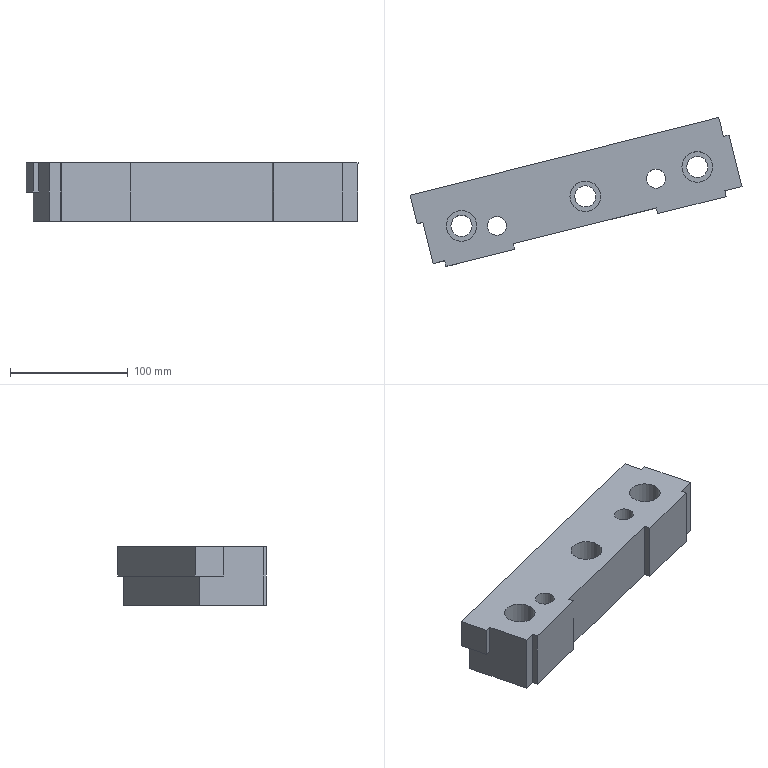Part | NX | features solid 2 | 1 solid | 31 faces | box 281.581 x 126.317 x 50 mm | volume 740203 mm3 | plane 20 | cylinder 8 | spline 3 | commonest cylinder face diameters 18 x3 26 x3 16 x2
STEP:
#1=CARTESIAN_POINT('',(-1.015,507.696,-50.));
#2=VERTEX_POINT('',#1);
#3=CARTESIAN_POINT('',(-10.015,507.696,-50.));
#4=DIRECTION('',(0.,0.,1.));
#5=DIRECTION('',(1.,0.,0.));
#6=AXIS2_PLACEMENT_3D('',#3,#4,#5);
#7=CIRCLE('',#6,9.);
#8=EDGE_CURVE('',#2,#2,#7,.T.);
#9=ORIENTED_EDGE('',*,*,#8,.F.);
#10=EDGE_LOOP('',(#9));
#11=FACE_BOUND('',#10,.T.);
#12=CARTESIAN_POINT('',(-1.015,507.696,-30.));
#13=VERTEX_POINT('',#12);
#14=CARTESIAN_POINT('',(-10.015,507.696,-30.));
#15=DIRECTION('',(0.,0.,1.));
#16=DIRECTION('',(1.,0.,0.));
#17=AXIS2_PLACEMENT_3D('',#14,#15,#16);
#18=CIRCLE('',#17,9.);
#19=EDGE_CURVE('',#13,#13,#18,.F.);
#20=ORIENTED_EDGE('',*,*,#19,.F.);
#21=EDGE_LOOP('',(#20));
#22=FACE_BOUND('',#21,.T.);
#23=CARTESIAN_POINT('',(-10.015,507.696,-125.));
#24=DIRECTION('',(0.,0.,1.));
#25=DIRECTION('',(1.,0.,0.));
#26=AXIS2_PLACEMENT_3D('',#23,#24,#25);
#27=CYLINDRICAL_SURFACE('',#26,9.);
#28=ADVANCED_FACE('',(#11,#22),#27,.F.);
#29=CARTESIAN_POINT('',(103.985,532.696,-50.));
#30=VERTEX_POINT('',#29);
#31=CARTESIAN_POINT('',(94.985,532.696,-50.));
#32=DIRECTION('',(0.,0.,1.));
#33=DIRECTION('',(1.,0.,0.));
#34=AXIS2_PLACEMENT_3D('',#31,#32,#33);
#35=CIRCLE('',#34,9.);
#36=EDGE_CURVE('',#30,#30,#35,.T.);
#37=ORIENTED_EDGE('',*,*,#36,.F.);
#38=EDGE_LOOP('',(#37));
#39=FACE_BOUND('',#38,.T.);
#40=CARTESIAN_POINT('',(103.985,532.696,-30.));
#41=VERTEX_POINT('',#40);
#42=CARTESIAN_POINT('',(94.985,532.696,-30.));
#43=DIRECTION('',(0.,0.,1.));
#44=DIRECTION('',(1.,0.,0.));
#45=AXIS2_PLACEMENT_3D('',#42,#43,#44);
#46=CIRCLE('',#45,9.);
#47=EDGE_CURVE('',#41,#41,#46,.F.);
#48=ORIENTED_EDGE('',*,*,#47,.F.);
#49=EDGE_LOOP('',(#48));
#50=FACE_BOUND('',#49,.T.);
#51=CARTESIAN_POINT('',(94.985,532.696,-125.));
#52=DIRECTION('',(0.,0.,1.));
#53=DIRECTION('',(1.,0.,0.));
#54=AXIS2_PLACEMENT_3D('',#51,#52,#53);
#55=CYLINDRICAL_SURFACE('',#54,9.);
#56=ADVANCED_FACE('',(#39,#50),#55,.F.);
#57=CARTESIAN_POINT('',(198.985,557.696,-50.));
#58=VERTEX_POINT('',#57);
#59=CARTESIAN_POINT('',(189.985,557.696,-50.));
#60=DIRECTION('',(0.,0.,1.));
#61=DIRECTION('',(1.,0.,0.));
#62=AXIS2_PLACEMENT_3D('',#59,#60,#61);
#63=CIRCLE('',#62,9.);
#64=EDGE_CURVE('',#58,#58,#63,.T.);
#65=ORIENTED_EDGE('',*,*,#64,.F.);
#66=EDGE_LOOP('',(#65));
#67=FACE_BOUND('',#66,.T.);
#68=CARTESIAN_POINT('',(198.985,557.696,-30.));
#69=VERTEX_POINT('',#68);
#70=CARTESIAN_POINT('',(189.985,557.696,-30.));
#71=DIRECTION('',(0.,0.,1.));
#72=DIRECTION('',(1.,0.,0.));
#73=AXIS2_PLACEMENT_3D('',#70,#71,#72);
#74=CIRCLE('',#73,9.);
#75=EDGE_CURVE('',#69,#69,#74,.F.);
#76=ORIENTED_EDGE('',*,*,#75,.F.);
#77=EDGE_LOOP('',(#76));
#78=FACE_BOUND('',#77,.T.);
#79=CARTESIAN_POINT('',(189.985,557.696,-125.));
#80=DIRECTION('',(0.,0.,1.));
#81=DIRECTION('',(1.,0.,0.));
#82=AXIS2_PLACEMENT_3D('',#79,#80,#81);
#83=CYLINDRICAL_SURFACE('',#82,9.);
#84=ADVANCED_FACE('',(#67,#78),#83,.F.);
#85=CARTESIAN_POINT('',(155.109,522.891,0.));
#86=VERTEX_POINT('',#85);
#87=CARTESIAN_POINT('',(155.109,522.891,-50.));
#88=VERTEX_POINT('',#87);
#89=CARTESIAN_POINT('',(155.109,522.891,-70.));
#90=DIRECTION('',(0.,0.,-1.));
#91=VECTOR('',#90,1000.);
#92=LINE('',#89,#91);
#93=EDGE_CURVE('',#86,#88,#92,.T.);
#94=ORIENTED_EDGE('',*,*,#93,.F.);
#95=CARTESIAN_POINT('',(33.822,492.651,0.));
#96=VERTEX_POINT('',#95);
#97=CARTESIAN_POINT('',(-300.93,409.188,0.));
#98=DIRECTION('',(-0.9703,-0.2419,0.));
#99=VECTOR('',#98,1000.);
#100=LINE('',#97,#99);
#101=EDGE_CURVE('',#86,#96,#100,.T.);
#102=ORIENTED_EDGE('',*,*,#101,.T.);
#103=CARTESIAN_POINT('',(33.822,492.651,-50.));
#104=VERTEX_POINT('',#103);
#105=CARTESIAN_POINT('',(33.822,492.651,-70.));
#106=DIRECTION('',(0.,0.,-1.));
#107=VECTOR('',#106,1000.);
#108=LINE('',#105,#107);
#109=EDGE_CURVE('',#96,#104,#108,.T.);
#110=ORIENTED_EDGE('',*,*,#109,.T.);
#111=CARTESIAN_POINT('',(-232.339,426.29,-50.));
#112=DIRECTION('',(0.9703,0.2419,0.));
#113=VECTOR('',#112,1000.);
#114=LINE('',#111,#113);
#115=EDGE_CURVE('',#104,#88,#114,.T.);
#116=ORIENTED_EDGE('',*,*,#115,.T.);
#117=EDGE_LOOP('',(#94,#102,#110,#116));
#118=FACE_BOUND('',#117,.T.);
#119=CARTESIAN_POINT('',(-300.93,409.188,-70.));
#120=DIRECTION('',(0.2419,-0.9703,0.));
#121=DIRECTION('',(0.9703,0.2419,0.));
#122=AXIS2_PLACEMENT_3D('',#119,#120,#121);
#123=PLANE('',#122);
#124=ADVANCED_FACE('',(#118),#123,.T.);
#125=CARTESIAN_POINT('',(212.143,583.489,0.));
#126=VERTEX_POINT('',#125);
#127=CARTESIAN_POINT('',(216.994,584.699,0.));
#128=VERTEX_POINT('',#127);
#129=CARTESIAN_POINT('',(212.143,583.489,0.));
#130=DIRECTION('',(0.9703,0.2419,0.));
#131=VECTOR('',#130,1000.);
#132=LINE('',#129,#131);
#133=EDGE_CURVE('',#126,#128,#132,.T.);
#134=ORIENTED_EDGE('',*,*,#133,.F.);
#135=CARTESIAN_POINT('',(208.125,599.602,0.));
#136=VERTEX_POINT('',#135);
#137=CARTESIAN_POINT('',(537.993,-723.425,0.));
#138=DIRECTION('',(-0.2419,0.9703,0.));
#139=VECTOR('',#138,1000.);
#140=LINE('',#137,#139);
#141=EDGE_CURVE('',#126,#136,#140,.T.);
#142=ORIENTED_EDGE('',*,*,#141,.T.);
#143=CARTESIAN_POINT('',(-53.7,533.663,0.));
#144=VERTEX_POINT('',#143);
#145=CARTESIAN_POINT('',(208.125,599.602,0.));
#146=CARTESIAN_POINT('',(120.85,577.623,0.));
#147=CARTESIAN_POINT('',(33.576,555.638,0.));
#148=CARTESIAN_POINT('',(-53.7,533.663,0.));
#149=B_SPLINE_CURVE_WITH_KNOTS('',3,(#145,#146,#147,#148),.UNSPECIFIED.,.F.,.F.,(4,4),(1.862,2.132),.UNSPECIFIED.);
#150=EDGE_CURVE('',#144,#136,#149,.F.);
#151=ORIENTED_EDGE('',*,*,#150,.F.);
#152=CARTESIAN_POINT('',(-47.652,509.406,0.));
#153=VERTEX_POINT('',#152);
#154=CARTESIAN_POINT('',(276.013,-788.744,0.));
#155=DIRECTION('',(-0.2419,0.9703,0.));
#156=VECTOR('',#155,1000.);
#157=LINE('',#154,#156);
#158=EDGE_CURVE('',#153,#144,#157,.T.);
#159=ORIENTED_EDGE('',*,*,#158,.F.);
#160=CARTESIAN_POINT('',(-42.803,510.627,0.));
#161=VERTEX_POINT('',#160);
#162=CARTESIAN_POINT('',(-47.652,509.406,0.));
#163=CARTESIAN_POINT('',(-46.036,509.813,0.));
#164=CARTESIAN_POINT('',(-44.419,510.22,0.));
#165=CARTESIAN_POINT('',(-42.803,510.627,0.));
#166=B_SPLINE_CURVE_WITH_KNOTS('',3,(#162,#163,#164,#165),.UNSPECIFIED.,.F.,.F.,(4,4),(0.,0.005),.UNSPECIFIED.);
#167=EDGE_CURVE('',#153,#161,#166,.T.);
#168=ORIENTED_EDGE('',*,*,#167,.T.);
#169=CARTESIAN_POINT('',(-34.099,475.717,0.));
#170=VERTEX_POINT('',#169);
#171=CARTESIAN_POINT('',(-23.213,432.053,0.));
#172=DIRECTION('',(0.2419,-0.9703,0.));
#173=VECTOR('',#172,1000.);
#174=LINE('',#171,#173);
#175=EDGE_CURVE('',#161,#170,#174,.T.);
#176=ORIENTED_EDGE('',*,*,#175,.T.);
#177=CARTESIAN_POINT('',(-24.396,478.136,0.));
#178=VERTEX_POINT('',#177);
#179=CARTESIAN_POINT('',(-300.93,409.188,0.));
#180=DIRECTION('',(-0.9703,-0.2419,0.));
#181=VECTOR('',#180,1000.);
#182=LINE('',#179,#181);
#183=EDGE_CURVE('',#178,#170,#182,.T.);
#184=ORIENTED_EDGE('',*,*,#183,.F.);
#185=CARTESIAN_POINT('',(-23.187,473.284,0.));
#186=VERTEX_POINT('',#185);
#187=CARTESIAN_POINT('',(-39.146,537.292,0.));
#188=DIRECTION('',(0.2419,-0.9703,0.));
#189=VECTOR('',#188,1000.);
#190=LINE('',#187,#189);
#191=EDGE_CURVE('',#178,#186,#190,.T.);
#192=ORIENTED_EDGE('',*,*,#191,.T.);
#193=CARTESIAN_POINT('',(35.031,487.8,0.));
#194=VERTEX_POINT('',#193);
#195=CARTESIAN_POINT('',(-231.129,421.438,0.));
#196=DIRECTION('',(0.9703,0.2419,0.));
#197=VECTOR('',#196,1000.);
#198=LINE('',#195,#197);
#199=EDGE_CURVE('',#186,#194,#198,.T.);
#200=ORIENTED_EDGE('',*,*,#199,.T.);
#201=CARTESIAN_POINT('',(19.072,551.808,0.));
#202=DIRECTION('',(0.2419,-0.9703,0.));
#203=VECTOR('',#202,1000.);
#204=LINE('',#201,#203);
#205=EDGE_CURVE('',#96,#194,#204,.T.);
#206=ORIENTED_EDGE('',*,*,#205,.F.);
#207=ORIENTED_EDGE('',*,*,#101,.F.);
#208=CARTESIAN_POINT('',(156.318,518.04,0.));
#209=VERTEX_POINT('',#208);
#210=CARTESIAN_POINT('',(140.359,582.048,0.));
#211=DIRECTION('',(0.2419,-0.9703,0.));
#212=VECTOR('',#211,1000.);
#213=LINE('',#210,#212);
#214=EDGE_CURVE('',#86,#209,#213,.T.);
#215=ORIENTED_EDGE('',*,*,#214,.T.);
#216=CARTESIAN_POINT('',(214.536,532.555,0.));
#217=VERTEX_POINT('',#216);
#218=CARTESIAN_POINT('',(-231.129,421.438,0.));
#219=DIRECTION('',(0.9703,0.2419,0.));
#220=VECTOR('',#219,1000.);
#221=LINE('',#218,#220);
#222=EDGE_CURVE('',#209,#217,#221,.T.);
#223=ORIENTED_EDGE('',*,*,#222,.T.);
#224=CARTESIAN_POINT('',(213.326,537.407,0.));
#225=VERTEX_POINT('',#224);
#226=CARTESIAN_POINT('',(198.577,596.563,0.));
#227=DIRECTION('',(0.2419,-0.9703,0.));
#228=VECTOR('',#227,1000.);
#229=LINE('',#226,#228);
#230=EDGE_CURVE('',#225,#217,#229,.T.);
#231=ORIENTED_EDGE('',*,*,#230,.F.);
#232=CARTESIAN_POINT('',(227.881,541.035,0.));
#233=VERTEX_POINT('',#232);
#234=CARTESIAN_POINT('',(-232.339,426.29,0.));
#235=DIRECTION('',(-0.9703,-0.2419,0.));
#236=VECTOR('',#235,1000.);
#237=LINE('',#234,#236);
#238=EDGE_CURVE('',#233,#225,#237,.T.);
#239=ORIENTED_EDGE('',*,*,#238,.F.);
#240=CARTESIAN_POINT('',(237.558,502.224,0.));
#241=DIRECTION('',(-0.2419,0.9703,0.));
#242=VECTOR('',#241,1000.);
#243=LINE('',#240,#242);
#244=EDGE_CURVE('',#233,#128,#243,.T.);
#245=ORIENTED_EDGE('',*,*,#244,.T.);
#246=EDGE_LOOP('',(#134,#142,#151,#159,#168,#176,#184,#192,#200,#206,#207,#215,#223,#231,#239,#245));
#247=FACE_BOUND('',#246,.T.);
#248=CARTESIAN_POINT('',(2.985,507.696,0.));
#249=VERTEX_POINT('',#248);
#250=CARTESIAN_POINT('',(-10.015,507.696,0.));
#251=DIRECTION('',(0.,0.,1.));
#252=DIRECTION('',(1.,0.,0.));
#253=AXIS2_PLACEMENT_3D('',#250,#251,#252);
#254=CIRCLE('',#253,13.);
#255=EDGE_CURVE('',#249,#249,#254,.T.);
#256=ORIENTED_EDGE('',*,*,#255,.F.);
#257=EDGE_LOOP('',(#256));
#258=FACE_BOUND('',#257,.T.);
#259=CARTESIAN_POINT('',(107.985,532.696,0.));
#260=VERTEX_POINT('',#259);
#261=CARTESIAN_POINT('',(94.985,532.696,0.));
#262=DIRECTION('',(0.,0.,1.));
#263=DIRECTION('',(1.,0.,0.));
#264=AXIS2_PLACEMENT_3D('',#261,#262,#263);
#265=CIRCLE('',#264,13.);
#266=EDGE_CURVE('',#260,#260,#265,.T.);
#267=ORIENTED_EDGE('',*,*,#266,.F.);
#268=EDGE_LOOP('',(#267));
#269=FACE_BOUND('',#268,.T.);
#270=CARTESIAN_POINT('',(202.985,557.696,0.));
#271=VERTEX_POINT('',#270);
#272=CARTESIAN_POINT('',(189.985,557.696,0.));
#273=DIRECTION('',(0.,0.,1.));
#274=DIRECTION('',(1.,0.,0.));
#275=AXIS2_PLACEMENT_3D('',#272,#273,#274);
#276=CIRCLE('',#275,13.);
#277=EDGE_CURVE('',#271,#271,#276,.T.);
#278=ORIENTED_EDGE('',*,*,#277,.F.);
#279=EDGE_LOOP('',(#278));
#280=FACE_BOUND('',#279,.T.);
#281=CARTESIAN_POINT('',(27.985,507.696,0.));
#282=VERTEX_POINT('',#281);
#283=CARTESIAN_POINT('',(19.985,507.696,0.));
#284=DIRECTION('',(0.,0.,1.));
#285=DIRECTION('',(1.,0.,0.));
#286=AXIS2_PLACEMENT_3D('',#283,#284,#285);
#287=CIRCLE('',#286,8.);
#288=EDGE_CURVE('',#282,#282,#287,.T.);
#289=ORIENTED_EDGE('',*,*,#288,.F.);
#290=EDGE_LOOP('',(#289));
#291=FACE_BOUND('',#290,.T.);
#292=CARTESIAN_POINT('',(162.985,547.696,0.));
#293=VERTEX_POINT('',#292);
#294=CARTESIAN_POINT('',(154.985,547.696,0.));
#295=DIRECTION('',(0.,0.,1.));
#296=DIRECTION('',(1.,0.,0.));
#297=AXIS2_PLACEMENT_3D('',#294,#295,#296);
#298=CIRCLE('',#297,8.);
#299=EDGE_CURVE('',#293,#293,#298,.T.);
#300=ORIENTED_EDGE('',*,*,#299,.F.);
#301=EDGE_LOOP('',(#300));
#302=FACE_BOUND('',#301,.T.);
#303=CARTESIAN_POINT('',(82.625,-836.961,0.));
#304=DIRECTION('',(0.,0.,1.));
#305=DIRECTION('',(1.,0.,0.));
#306=AXIS2_PLACEMENT_3D('',#303,#304,#305);
#307=PLANE('',#306);
#308=ADVANCED_FACE('',(#247,#258,#269,#280,#291,#302),#307,.T.);
#309=CARTESIAN_POINT('',(-47.652,509.406,-25.));
#310=VERTEX_POINT('',#309);
#311=CARTESIAN_POINT('',(-42.803,510.627,-25.));
#312=VERTEX_POINT('',#311);
#313=CARTESIAN_POINT('',(-47.652,509.406,-25.));
#314=CARTESIAN_POINT('',(-46.036,509.813,-25.));
#315=CARTESIAN_POINT('',(-44.419,510.22,-25.));
#316=CARTESIAN_POINT('',(-42.803,510.627,-25.));
#317=B_SPLINE_CURVE_WITH_KNOTS('',3,(#313,#314,#315,#316),.UNSPECIFIED.,.F.,.F.,(4,4),(-0.0002137,0.01831),.UNSPECIFIED.);
#318=EDGE_CURVE('',#310,#312,#317,.T.);
#319=ORIENTED_EDGE('',*,*,#318,.F.);
#320=CARTESIAN_POINT('',(-53.7,533.663,-25.));
#321=VERTEX_POINT('',#320);
#322=CARTESIAN_POINT('',(-53.7,533.663,-25.));
#323=DIRECTION('',(0.2419,-0.9703,0.));
#324=VECTOR('',#323,1000.);
#325=LINE('',#322,#324);
#326=EDGE_CURVE('',#321,#310,#325,.T.);
#327=ORIENTED_EDGE('',*,*,#326,.F.);
#328=CARTESIAN_POINT('',(208.125,599.602,-25.));
#329=VERTEX_POINT('',#328);
#330=CARTESIAN_POINT('',(208.125,599.602,-25.));
#331=CARTESIAN_POINT('',(120.85,577.623,-25.));
#332=CARTESIAN_POINT('',(33.576,555.638,-25.));
#333=CARTESIAN_POINT('',(-53.7,533.663,-25.));
#334=B_SPLINE_CURVE_WITH_KNOTS('',3,(#330,#331,#332,#333),.UNSPECIFIED.,.F.,.F.,(4,4),(1.907,2.177),.UNSPECIFIED.);
#335=EDGE_CURVE('',#321,#329,#334,.F.);
#336=ORIENTED_EDGE('',*,*,#335,.T.);
#337=CARTESIAN_POINT('',(209.335,594.75,-25.));
#338=VERTEX_POINT('',#337);
#339=CARTESIAN_POINT('',(820.536,-1856.645,-25.));
#340=DIRECTION('',(-0.2419,0.9703,0.));
#341=VECTOR('',#340,1000.);
#342=LINE('',#339,#341);
#343=EDGE_CURVE('',#338,#329,#342,.T.);
#344=ORIENTED_EDGE('',*,*,#343,.F.);
#345=CARTESIAN_POINT('',(-47.642,530.033,-25.));
#346=VERTEX_POINT('',#345);
#347=CARTESIAN_POINT('',(209.335,594.75,-25.));
#348=CARTESIAN_POINT('',(123.676,573.178,-25.));
#349=CARTESIAN_POINT('',(38.019,551.599,-25.));
#350=CARTESIAN_POINT('',(-47.642,530.033,-25.));
#351=B_SPLINE_CURVE_WITH_KNOTS('',3,(#347,#348,#349,#350),.UNSPECIFIED.,.F.,.F.,(4,4),(1.091,1.356),.UNSPECIFIED.);
#352=EDGE_CURVE('',#346,#338,#351,.F.);
#353=ORIENTED_EDGE('',*,*,#352,.F.);
#354=CARTESIAN_POINT('',(-23.213,432.053,-25.));
#355=DIRECTION('',(-0.2419,0.9703,0.));
#356=VECTOR('',#355,1000.);
#357=LINE('',#354,#356);
#358=EDGE_CURVE('',#312,#346,#357,.T.);
#359=ORIENTED_EDGE('',*,*,#358,.F.);
#360=EDGE_LOOP('',(#319,#327,#336,#344,#353,#359));
#361=FACE_BOUND('',#360,.T.);
#362=CARTESIAN_POINT('',(-53.7,533.663,-25.));
#363=DIRECTION('',(0.,0.,-1.));
#364=DIRECTION('',(-1.,0.,0.));
#365=AXIS2_PLACEMENT_3D('',#362,#363,#364);
#366=PLANE('',#365);
#367=ADVANCED_FACE('',(#361),#366,.T.);
#368=ORIENTED_EDGE('',*,*,#326,.T.);
#369=CARTESIAN_POINT('',(-47.652,509.406,-12.5));
#370=DIRECTION('',(0.,0.,-1.));
#371=VECTOR('',#370,1000.);
#372=LINE('',#369,#371);
#373=EDGE_CURVE('',#310,#153,#372,.F.);
#374=ORIENTED_EDGE('',*,*,#373,.T.);
#375=ORIENTED_EDGE('',*,*,#158,.T.);
#376=CARTESIAN_POINT('',(-53.7,533.663,-2.5));
#377=DIRECTION('',(0.,0.,1.));
#378=VECTOR('',#377,1000.);
#379=LINE('',#376,#378);
#380=EDGE_CURVE('',#321,#144,#379,.T.);
#381=ORIENTED_EDGE('',*,*,#380,.F.);
#382=EDGE_LOOP('',(#368,#374,#375,#381));
#383=FACE_BOUND('',#382,.T.);
#384=CARTESIAN_POINT('',(558.557,-1921.963,-70.));
#385=DIRECTION('',(0.9703,0.2419,0.));
#386=DIRECTION('',(-0.2419,0.9703,0.));
#387=AXIS2_PLACEMENT_3D('',#384,#385,#386);
#388=PLANE('',#387);
#389=ADVANCED_FACE('',(#383),#388,.F.);
#390=CARTESIAN_POINT('',(-24.396,478.136,-50.));
#391=VERTEX_POINT('',#390);
#392=CARTESIAN_POINT('',(-24.396,478.136,-70.));
#393=DIRECTION('',(0.,0.,-1.));
#394=VECTOR('',#393,1000.);
#395=LINE('',#392,#394);
#396=EDGE_CURVE('',#178,#391,#395,.T.);
#397=ORIENTED_EDGE('',*,*,#396,.F.);
#398=ORIENTED_EDGE('',*,*,#183,.T.);
#399=CARTESIAN_POINT('',(-34.099,475.717,-50.));
#400=VERTEX_POINT('',#399);
#401=CARTESIAN_POINT('',(-34.099,475.717,-70.));
#402=DIRECTION('',(0.,0.,1.));
#403=VECTOR('',#402,1000.);
#404=LINE('',#401,#403);
#405=EDGE_CURVE('',#400,#170,#404,.T.);
#406=ORIENTED_EDGE('',*,*,#405,.F.);
#407=CARTESIAN_POINT('',(-232.339,426.29,-50.));
#408=DIRECTION('',(0.9703,0.2419,0.));
#409=VECTOR('',#408,1000.);
#410=LINE('',#407,#409);
#411=EDGE_CURVE('',#400,#391,#410,.T.);
#412=ORIENTED_EDGE('',*,*,#411,.T.);
#413=EDGE_LOOP('',(#397,#398,#406,#412));
#414=FACE_BOUND('',#413,.T.);
#415=CARTESIAN_POINT('',(-300.93,409.188,-70.));
#416=DIRECTION('',(0.2419,-0.9703,0.));
#417=DIRECTION('',(0.9703,0.2419,0.));
#418=AXIS2_PLACEMENT_3D('',#415,#416,#417);
#419=PLANE('',#418);
#420=ADVANCED_FACE('',(#414),#419,.T.);
#421=CARTESIAN_POINT('',(212.143,583.489,-50.));
#422=VERTEX_POINT('',#421);
#423=CARTESIAN_POINT('',(212.143,583.489,-70.));
#424=DIRECTION('',(0.,0.,1.));
#425=VECTOR('',#424,1000.);
#426=LINE('',#423,#425);
#427=EDGE_CURVE('',#422,#126,#426,.T.);
#428=ORIENTED_EDGE('',*,*,#427,.F.);
#429=CARTESIAN_POINT('',(209.335,594.75,-50.));
#430=VERTEX_POINT('',#429);
#431=CARTESIAN_POINT('',(537.993,-723.425,-50.));
#432=DIRECTION('',(-0.2419,0.9703,0.));
#433=VECTOR('',#432,1000.);
#434=LINE('',#431,#433);
#435=EDGE_CURVE('',#422,#430,#434,.T.);
#436=ORIENTED_EDGE('',*,*,#435,.T.);
#437=CARTESIAN_POINT('',(209.335,594.75,-42.5));
#438=DIRECTION('',(0.,0.,1.));
#439=VECTOR('',#438,1000.);
#440=LINE('',#437,#439);
#441=EDGE_CURVE('',#338,#430,#440,.F.);
#442=ORIENTED_EDGE('',*,*,#441,.F.);
#443=ORIENTED_EDGE('',*,*,#343,.T.);
#444=CARTESIAN_POINT('',(208.125,599.602,-70.));
#445=DIRECTION('',(0.,0.,1.));
#446=VECTOR('',#445,1000.);
#447=LINE('',#444,#446);
#448=EDGE_CURVE('',#329,#136,#447,.T.);
#449=ORIENTED_EDGE('',*,*,#448,.T.);
#450=ORIENTED_EDGE('',*,*,#141,.F.);
#451=EDGE_LOOP('',(#428,#436,#442,#443,#449,#450));
#452=FACE_BOUND('',#451,.T.);
#453=CARTESIAN_POINT('',(820.536,-1856.645,-70.));
#454=DIRECTION('',(0.9703,0.2419,0.));
#455=DIRECTION('',(-0.2419,0.9703,0.));
#456=AXIS2_PLACEMENT_3D('',#453,#454,#455);
#457=PLANE('',#456);
#458=ADVANCED_FACE('',(#452),#457,.T.);
#459=ORIENTED_EDGE('',*,*,#175,.F.);
#460=CARTESIAN_POINT('',(-42.803,510.627,-25.));
#461=DIRECTION('',(0.,0.,-1.));
#462=VECTOR('',#461,1000.);
#463=LINE('',#460,#462);
#464=EDGE_CURVE('',#312,#161,#463,.F.);
#465=ORIENTED_EDGE('',*,*,#464,.F.);
#466=ORIENTED_EDGE('',*,*,#358,.T.);
#467=CARTESIAN_POINT('',(-47.642,530.033,-50.));
#468=VERTEX_POINT('',#467);
#469=CARTESIAN_POINT('',(-47.642,530.033,-42.5));
#470=DIRECTION('',(0.,0.,1.));
#471=VECTOR('',#470,1000.);
#472=LINE('',#469,#471);
#473=EDGE_CURVE('',#468,#346,#472,.T.);
#474=ORIENTED_EDGE('',*,*,#473,.F.);
#475=CARTESIAN_POINT('',(280.865,-787.534,-50.));
#476=DIRECTION('',(-0.2419,0.9703,0.));
#477=VECTOR('',#476,1000.);
#478=LINE('',#475,#477);
#479=EDGE_CURVE('',#400,#468,#478,.T.);
#480=ORIENTED_EDGE('',*,*,#479,.F.);
#481=ORIENTED_EDGE('',*,*,#405,.T.);
#482=EDGE_LOOP('',(#459,#465,#466,#474,#480,#481));
#483=FACE_BOUND('',#482,.T.);
#484=CARTESIAN_POINT('',(-23.213,432.053,-70.));
#485=DIRECTION('',(0.9703,0.2419,0.));
#486=DIRECTION('',(-0.2419,0.9703,0.));
#487=AXIS2_PLACEMENT_3D('',#484,#485,#486);
#488=PLANE('',#487);
#489=ADVANCED_FACE('',(#483),#488,.F.);
#490=ORIENTED_EDGE('',*,*,#8,.T.);
#491=EDGE_LOOP('',(#490));
#492=FACE_BOUND('',#491,.T.);
#493=CARTESIAN_POINT('',(27.985,507.696,-50.));
#494=VERTEX_POINT('',#493);
#495=CARTESIAN_POINT('',(19.985,507.696,-50.));
#496=DIRECTION('',(0.,0.,1.));
#497=DIRECTION('',(1.,0.,0.));
#498=AXIS2_PLACEMENT_3D('',#495,#496,#497);
#499=CIRCLE('',#498,8.);
#500=EDGE_CURVE('',#494,#494,#499,.T.);
#501=ORIENTED_EDGE('',*,*,#500,.T.);
#502=EDGE_LOOP('',(#501));
#503=FACE_BOUND('',#502,.T.);
#504=ORIENTED_EDGE('',*,*,#36,.T.);
#505=EDGE_LOOP('',(#504));
#506=FACE_BOUND('',#505,.T.);
#507=CARTESIAN_POINT('',(162.985,547.696,-50.));
#508=VERTEX_POINT('',#507);
#509=CARTESIAN_POINT('',(154.985,547.696,-50.));
#510=DIRECTION('',(0.,0.,1.));
#511=DIRECTION('',(1.,0.,0.));
#512=AXIS2_PLACEMENT_3D('',#509,#510,#511);
#513=CIRCLE('',#512,8.);
#514=EDGE_CURVE('',#508,#508,#513,.T.);
#515=ORIENTED_EDGE('',*,*,#514,.T.);
#516=EDGE_LOOP('',(#515));
#517=FACE_BOUND('',#516,.T.);
#518=ORIENTED_EDGE('',*,*,#64,.T.);
#519=EDGE_LOOP('',(#518));
#520=FACE_BOUND('',#519,.T.);
#521=ORIENTED_EDGE('',*,*,#479,.T.);
#522=CARTESIAN_POINT('',(-47.642,530.033,-50.));
#523=CARTESIAN_POINT('',(38.017,551.605,-50.));
#524=CARTESIAN_POINT('',(123.676,573.178,-50.));
#525=CARTESIAN_POINT('',(209.335,594.75,-50.));
#526=B_SPLINE_CURVE_WITH_KNOTS('',3,(#522,#523,#524,#525),.UNSPECIFIED.,.F.,.F.,(4,4),(0.,1.),.UNSPECIFIED.);
#527=EDGE_CURVE('',#468,#430,#526,.T.);
#528=ORIENTED_EDGE('',*,*,#527,.T.);
#529=ORIENTED_EDGE('',*,*,#435,.F.);
#530=CARTESIAN_POINT('',(216.994,584.699,-50.));
#531=VERTEX_POINT('',#530);
#532=CARTESIAN_POINT('',(212.143,583.489,-50.));
#533=DIRECTION('',(0.9703,0.2419,0.));
#534=VECTOR('',#533,1000.);
#535=LINE('',#532,#534);
#536=EDGE_CURVE('',#422,#531,#535,.T.);
#537=ORIENTED_EDGE('',*,*,#536,.T.);
#538=CARTESIAN_POINT('',(227.881,541.035,-50.));
#539=VERTEX_POINT('',#538);
#540=CARTESIAN_POINT('',(237.558,502.224,-50.));
#541=DIRECTION('',(-0.2419,0.9703,0.));
#542=VECTOR('',#541,1000.);
#543=LINE('',#540,#542);
#544=EDGE_CURVE('',#539,#531,#543,.T.);
#545=ORIENTED_EDGE('',*,*,#544,.F.);
#546=CARTESIAN_POINT('',(213.326,537.407,-50.));
#547=VERTEX_POINT('',#546);
#548=CARTESIAN_POINT('',(223.029,539.826,-50.));
#549=DIRECTION('',(0.9703,0.2419,0.));
#550=VECTOR('',#549,1000.);
#551=LINE('',#548,#550);
#552=EDGE_CURVE('',#547,#539,#551,.T.);
#553=ORIENTED_EDGE('',*,*,#552,.F.);
#554=CARTESIAN_POINT('',(214.536,532.555,-50.));
#555=VERTEX_POINT('',#554);
#556=CARTESIAN_POINT('',(218.165,518.001,-50.));
#557=DIRECTION('',(0.2419,-0.9703,0.));
#558=VECTOR('',#557,1000.);
#559=LINE('',#556,#558);
#560=EDGE_CURVE('',#547,#555,#559,.T.);
#561=ORIENTED_EDGE('',*,*,#560,.T.);
#562=CARTESIAN_POINT('',(156.318,518.04,-50.));
#563=VERTEX_POINT('',#562);
#564=CARTESIAN_POINT('',(-231.129,421.438,-50.));
#565=DIRECTION('',(0.9703,0.2419,0.));
#566=VECTOR('',#565,1000.);
#567=LINE('',#564,#566);
#568=EDGE_CURVE('',#563,#555,#567,.T.);
#569=ORIENTED_EDGE('',*,*,#568,.F.);
#570=CARTESIAN_POINT('',(159.947,503.485,-50.));
#571=DIRECTION('',(0.2419,-0.9703,0.));
#572=VECTOR('',#571,1000.);
#573=LINE('',#570,#572);
#574=EDGE_CURVE('',#88,#563,#573,.T.);
#575=ORIENTED_EDGE('',*,*,#574,.F.);
#576=ORIENTED_EDGE('',*,*,#115,.F.);
#577=CARTESIAN_POINT('',(35.031,487.8,-50.));
#578=VERTEX_POINT('',#577);
#579=CARTESIAN_POINT('',(38.66,473.245,-50.));
#580=DIRECTION('',(0.2419,-0.9703,0.));
#581=VECTOR('',#580,1000.);
#582=LINE('',#579,#581);
#583=EDGE_CURVE('',#104,#578,#582,.T.);
#584=ORIENTED_EDGE('',*,*,#583,.T.);
#585=CARTESIAN_POINT('',(-23.187,473.284,-50.));
#586=VERTEX_POINT('',#585);
#587=CARTESIAN_POINT('',(-231.129,421.438,-50.));
#588=DIRECTION('',(0.9703,0.2419,0.));
#589=VECTOR('',#588,1000.);
#590=LINE('',#587,#589);
#591=EDGE_CURVE('',#586,#578,#590,.T.);
#592=ORIENTED_EDGE('',*,*,#591,.F.);
#593=CARTESIAN_POINT('',(-19.558,458.73,-50.));
#594=DIRECTION('',(0.2419,-0.9703,0.));
#595=VECTOR('',#594,1000.);
#596=LINE('',#593,#595);
#597=EDGE_CURVE('',#391,#586,#596,.T.);
#598=ORIENTED_EDGE('',*,*,#597,.F.);
#599=ORIENTED_EDGE('',*,*,#411,.F.);
#600=EDGE_LOOP('',(#521,#528,#529,#537,#545,#553,#561,#569,#575,#576,#584,#592,#598,#599));
#601=FACE_BOUND('',#600,.T.);
#602=CARTESIAN_POINT('',(82.625,-836.961,-50.));
#603=DIRECTION('',(0.,0.,1.));
#604=DIRECTION('',(1.,0.,0.));
#605=AXIS2_PLACEMENT_3D('',#602,#603,#604);
#606=PLANE('',#605);
#607=ADVANCED_FACE('',(#492,#503,#506,#517,#520,#601),#606,.F.);
#608=ORIENTED_EDGE('',*,*,#335,.F.);
#609=ORIENTED_EDGE('',*,*,#380,.T.);
#610=ORIENTED_EDGE('',*,*,#150,.T.);
#611=ORIENTED_EDGE('',*,*,#448,.F.);
#612=EDGE_LOOP('',(#608,#609,#610,#611));
#613=FACE_BOUND('',#612,.T.);
#614=CARTESIAN_POINT('',(-53.7,533.663,-25.));
#615=CARTESIAN_POINT('',(-53.7,533.663,0.));
#616=CARTESIAN_POINT('',(33.576,555.638,-25.));
#617=CARTESIAN_POINT('',(33.576,555.638,0.));
#618=CARTESIAN_POINT('',(120.85,577.623,-25.));
#619=CARTESIAN_POINT('',(120.85,577.623,0.));
#620=CARTESIAN_POINT('',(208.125,599.602,-25.));
#621=CARTESIAN_POINT('',(208.125,599.602,0.));
#622=B_SPLINE_SURFACE_WITH_KNOTS('',3,1,((#614,#615),(#616,#617),(#618,#619),(#620,#621)),.SURF_OF_LINEAR_EXTRUSION.,.F.,.F.,.F.,(4,4),(2,2),(0.7681,0.9986),(0.,1.),.PIECEWISE_BEZIER_KNOTS.);
#623=ADVANCED_FACE('',(#613),#622,.F.);
#624=ORIENTED_EDGE('',*,*,#527,.F.);
#625=ORIENTED_EDGE('',*,*,#473,.T.);
#626=ORIENTED_EDGE('',*,*,#352,.T.);
#627=ORIENTED_EDGE('',*,*,#441,.T.);
#628=EDGE_LOOP('',(#624,#625,#626,#627));
#629=FACE_BOUND('',#628,.T.);
#630=CARTESIAN_POINT('',(-47.642,530.033,-50.));
#631=CARTESIAN_POINT('',(-47.642,530.033,-25.));
#632=CARTESIAN_POINT('',(38.018,551.599,-50.));
#633=CARTESIAN_POINT('',(38.018,551.599,-25.));
#634=CARTESIAN_POINT('',(123.676,573.178,-50.));
#635=CARTESIAN_POINT('',(123.676,573.178,-25.));
#636=CARTESIAN_POINT('',(209.335,594.75,-50.));
#637=CARTESIAN_POINT('',(209.335,594.75,-25.));
#638=B_SPLINE_SURFACE_WITH_KNOTS('',3,1,((#630,#631),(#632,#633),(#634,#635),(#636,#637)),.SURF_OF_LINEAR_EXTRUSION.,.F.,.F.,.F.,(4,4),(2,2),(0.01848,1.),(0.,1.),.PIECEWISE_BEZIER_KNOTS.);
#639=ADVANCED_FACE('',(#629),#638,.F.);
#640=ORIENTED_EDGE('',*,*,#464,.T.);
#641=ORIENTED_EDGE('',*,*,#167,.F.);
#642=ORIENTED_EDGE('',*,*,#373,.F.);
#643=ORIENTED_EDGE('',*,*,#318,.T.);
#644=EDGE_LOOP('',(#640,#641,#642,#643));
#645=FACE_BOUND('',#644,.T.);
#646=CARTESIAN_POINT('',(-47.652,509.406,0.));
#647=CARTESIAN_POINT('',(-47.652,509.406,-25.));
#648=CARTESIAN_POINT('',(-46.036,509.813,0.));
#649=CARTESIAN_POINT('',(-46.036,509.813,-25.));
#650=CARTESIAN_POINT('',(-44.419,510.22,0.));
#651=CARTESIAN_POINT('',(-44.419,510.22,-25.));
#652=CARTESIAN_POINT('',(-42.803,510.627,0.));
#653=CARTESIAN_POINT('',(-42.803,510.627,-25.));
#654=B_SPLINE_SURFACE_WITH_KNOTS('',3,1,((#646,#647),(#648,#649),(#650,#651),(#652,#653)),.SURF_OF_LINEAR_EXTRUSION.,.F.,.F.,.F.,(4,4),(2,2),(-0.0002137,0.01831),(0.,1.),.PIECEWISE_BEZIER_KNOTS.);
#655=ADVANCED_FACE('',(#645),#654,.F.);
#656=CARTESIAN_POINT('',(216.994,584.699,-50.));
#657=DIRECTION('',(0.,0.,1.));
#658=VECTOR('',#657,1000.);
#659=LINE('',#656,#658);
#660=EDGE_CURVE('',#531,#128,#659,.T.);
#661=ORIENTED_EDGE('',*,*,#660,.F.);
#662=ORIENTED_EDGE('',*,*,#536,.F.);
#663=ORIENTED_EDGE('',*,*,#427,.T.);
#664=ORIENTED_EDGE('',*,*,#133,.T.);
#665=EDGE_LOOP('',(#661,#662,#663,#664));
#666=FACE_BOUND('',#665,.T.);
#667=CARTESIAN_POINT('',(212.143,583.489,-50.));
#668=DIRECTION('',(-0.2419,0.9703,0.));
#669=DIRECTION('',(-0.9703,-0.2419,0.));
#670=AXIS2_PLACEMENT_3D('',#667,#668,#669);
#671=PLANE('',#670);
#672=ADVANCED_FACE('',(#666),#671,.T.);
#673=CARTESIAN_POINT('',(227.881,541.035,-50.));
#674=DIRECTION('',(0.,0.,1.));
#675=VECTOR('',#674,1000.);
#676=LINE('',#673,#675);
#677=EDGE_CURVE('',#539,#233,#676,.T.);
#678=ORIENTED_EDGE('',*,*,#677,.T.);
#679=ORIENTED_EDGE('',*,*,#238,.T.);
#680=CARTESIAN_POINT('',(213.326,537.407,-25.));
#681=DIRECTION('',(0.,0.,-1.));
#682=VECTOR('',#681,1000.);
#683=LINE('',#680,#682);
#684=EDGE_CURVE('',#225,#547,#683,.T.);
#685=ORIENTED_EDGE('',*,*,#684,.T.);
#686=ORIENTED_EDGE('',*,*,#552,.T.);
#687=EDGE_LOOP('',(#678,#679,#685,#686));
#688=FACE_BOUND('',#687,.T.);
#689=CARTESIAN_POINT('',(223.029,539.826,-50.));
#690=DIRECTION('',(-0.2419,0.9703,0.));
#691=DIRECTION('',(-0.9703,-0.2419,0.));
#692=AXIS2_PLACEMENT_3D('',#689,#690,#691);
#693=PLANE('',#692);
#694=ADVANCED_FACE('',(#688),#693,.F.);
#695=ORIENTED_EDGE('',*,*,#660,.T.);
#696=ORIENTED_EDGE('',*,*,#244,.F.);
#697=ORIENTED_EDGE('',*,*,#677,.F.);
#698=ORIENTED_EDGE('',*,*,#544,.T.);
#699=EDGE_LOOP('',(#695,#696,#697,#698));
#700=FACE_BOUND('',#699,.T.);
#701=CARTESIAN_POINT('',(237.558,502.224,-50.));
#702=DIRECTION('',(-0.9703,-0.2419,0.));
#703=DIRECTION('',(0.,0.,1.));
#704=AXIS2_PLACEMENT_3D('',#701,#702,#703);
#705=PLANE('',#704);
#706=ADVANCED_FACE('',(#700),#705,.F.);
#707=CARTESIAN_POINT('',(35.031,487.8,-25.));
#708=DIRECTION('',(0.,0.,-1.));
#709=VECTOR('',#708,1000.);
#710=LINE('',#707,#709);
#711=EDGE_CURVE('',#194,#578,#710,.T.);
#712=ORIENTED_EDGE('',*,*,#711,.T.);
#713=ORIENTED_EDGE('',*,*,#583,.F.);
#714=ORIENTED_EDGE('',*,*,#109,.F.);
#715=ORIENTED_EDGE('',*,*,#205,.T.);
#716=EDGE_LOOP('',(#712,#713,#714,#715));
#717=FACE_BOUND('',#716,.T.);
#718=CARTESIAN_POINT('',(38.66,473.245,-25.));
#719=DIRECTION('',(-0.9703,-0.2419,0.));
#720=DIRECTION('',(0.2419,-0.9703,0.));
#721=AXIS2_PLACEMENT_3D('',#718,#719,#720);
#722=PLANE('',#721);
#723=ADVANCED_FACE('',(#717),#722,.F.);
#724=CARTESIAN_POINT('',(-23.187,473.284,-25.));
#725=DIRECTION('',(0.,0.,-1.));
#726=VECTOR('',#725,1000.);
#727=LINE('',#724,#726);
#728=EDGE_CURVE('',#186,#586,#727,.T.);
#729=ORIENTED_EDGE('',*,*,#728,.F.);
#730=ORIENTED_EDGE('',*,*,#191,.F.);
#731=ORIENTED_EDGE('',*,*,#396,.T.);
#732=ORIENTED_EDGE('',*,*,#597,.T.);
#733=EDGE_LOOP('',(#729,#730,#731,#732));
#734=FACE_BOUND('',#733,.T.);
#735=CARTESIAN_POINT('',(-19.558,458.73,-25.));
#736=DIRECTION('',(-0.9703,-0.2419,0.));
#737=DIRECTION('',(0.2419,-0.9703,0.));
#738=AXIS2_PLACEMENT_3D('',#735,#736,#737);
#739=PLANE('',#738);
#740=ADVANCED_FACE('',(#734),#739,.T.);
#741=ORIENTED_EDGE('',*,*,#711,.F.);
#742=ORIENTED_EDGE('',*,*,#199,.F.);
#743=ORIENTED_EDGE('',*,*,#728,.T.);
#744=ORIENTED_EDGE('',*,*,#591,.T.);
#745=EDGE_LOOP('',(#741,#742,#743,#744));
#746=FACE_BOUND('',#745,.T.);
#747=CARTESIAN_POINT('',(-32.89,470.865,-25.));
#748=DIRECTION('',(0.2419,-0.9703,0.));
#749=DIRECTION('',(0.,0.,-1.));
#750=AXIS2_PLACEMENT_3D('',#747,#748,#749);
#751=PLANE('',#750);
#752=ADVANCED_FACE('',(#746),#751,.T.);
#753=CARTESIAN_POINT('',(214.536,532.555,-25.));
#754=DIRECTION('',(0.,0.,-1.));
#755=VECTOR('',#754,1000.);
#756=LINE('',#753,#755);
#757=EDGE_CURVE('',#217,#555,#756,.T.);
#758=ORIENTED_EDGE('',*,*,#757,.T.);
#759=ORIENTED_EDGE('',*,*,#560,.F.);
#760=ORIENTED_EDGE('',*,*,#684,.F.);
#761=ORIENTED_EDGE('',*,*,#230,.T.);
#762=EDGE_LOOP('',(#758,#759,#760,#761));
#763=FACE_BOUND('',#762,.T.);
#764=CARTESIAN_POINT('',(218.165,518.001,-25.));
#765=DIRECTION('',(-0.9703,-0.2419,0.));
#766=DIRECTION('',(0.2419,-0.9703,0.));
#767=AXIS2_PLACEMENT_3D('',#764,#765,#766);
#768=PLANE('',#767);
#769=ADVANCED_FACE('',(#763),#768,.F.);
#770=CARTESIAN_POINT('',(156.318,518.04,-25.));
#771=DIRECTION('',(0.,0.,-1.));
#772=VECTOR('',#771,1000.);
#773=LINE('',#770,#772);
#774=EDGE_CURVE('',#209,#563,#773,.T.);
#775=ORIENTED_EDGE('',*,*,#774,.F.);
#776=ORIENTED_EDGE('',*,*,#214,.F.);
#777=ORIENTED_EDGE('',*,*,#93,.T.);
#778=ORIENTED_EDGE('',*,*,#574,.T.);
#779=EDGE_LOOP('',(#775,#776,#777,#778));
#780=FACE_BOUND('',#779,.T.);
#781=CARTESIAN_POINT('',(159.947,503.485,-25.));
#782=DIRECTION('',(-0.9703,-0.2419,0.));
#783=DIRECTION('',(0.2419,-0.9703,0.));
#784=AXIS2_PLACEMENT_3D('',#781,#782,#783);
#785=PLANE('',#784);
#786=ADVANCED_FACE('',(#780),#785,.T.);
#787=ORIENTED_EDGE('',*,*,#757,.F.);
#788=ORIENTED_EDGE('',*,*,#222,.F.);
#789=ORIENTED_EDGE('',*,*,#774,.T.);
#790=ORIENTED_EDGE('',*,*,#568,.T.);
#791=EDGE_LOOP('',(#787,#788,#789,#790));
#792=FACE_BOUND('',#791,.T.);
#793=CARTESIAN_POINT('',(175.724,522.878,-25.));
#794=DIRECTION('',(0.2419,-0.9703,0.));
#795=DIRECTION('',(0.,0.,-1.));
#796=AXIS2_PLACEMENT_3D('',#793,#794,#795);
#797=PLANE('',#796);
#798=ADVANCED_FACE('',(#792),#797,.T.);
#799=ORIENTED_EDGE('',*,*,#299,.T.);
#800=EDGE_LOOP('',(#799));
#801=FACE_BOUND('',#800,.T.);
#802=ORIENTED_EDGE('',*,*,#514,.F.);
#803=EDGE_LOOP('',(#802));
#804=FACE_BOUND('',#803,.T.);
#805=CARTESIAN_POINT('',(154.985,547.696,-125.));
#806=DIRECTION('',(0.,0.,1.));
#807=DIRECTION('',(1.,0.,0.));
#808=AXIS2_PLACEMENT_3D('',#805,#806,#807);
#809=CYLINDRICAL_SURFACE('',#808,8.);
#810=ADVANCED_FACE('',(#801,#804),#809,.F.);
#811=ORIENTED_EDGE('',*,*,#288,.T.);
#812=EDGE_LOOP('',(#811));
#813=FACE_BOUND('',#812,.T.);
#814=ORIENTED_EDGE('',*,*,#500,.F.);
#815=EDGE_LOOP('',(#814));
#816=FACE_BOUND('',#815,.T.);
#817=CARTESIAN_POINT('',(19.985,507.696,-125.));
#818=DIRECTION('',(0.,0.,1.));
#819=DIRECTION('',(1.,0.,0.));
#820=AXIS2_PLACEMENT_3D('',#817,#818,#819);
#821=CYLINDRICAL_SURFACE('',#820,8.);
#822=ADVANCED_FACE('',(#813,#816),#821,.F.);
#823=CARTESIAN_POINT('',(202.985,557.696,-30.));
#824=VERTEX_POINT('',#823);
#825=CARTESIAN_POINT('',(189.985,557.696,-30.));
#826=DIRECTION('',(0.,0.,1.));
#827=DIRECTION('',(1.,0.,0.));
#828=AXIS2_PLACEMENT_3D('',#825,#826,#827);
#829=CIRCLE('',#828,13.);
#830=EDGE_CURVE('',#824,#824,#829,.T.);
#831=ORIENTED_EDGE('',*,*,#830,.T.);
#832=EDGE_LOOP('',(#831));
#833=FACE_BOUND('',#832,.T.);
#834=ORIENTED_EDGE('',*,*,#75,.T.);
#835=EDGE_LOOP('',(#834));
#836=FACE_BOUND('',#835,.T.);
#837=CARTESIAN_POINT('',(189.985,557.696,-30.));
#838=DIRECTION('',(0.,0.,1.));
#839=DIRECTION('',(1.,0.,0.));
#840=AXIS2_PLACEMENT_3D('',#837,#838,#839);
#841=PLANE('',#840);
#842=ADVANCED_FACE('',(#833,#836),#841,.T.);
#843=ORIENTED_EDGE('',*,*,#830,.F.);
#844=EDGE_LOOP('',(#843));
#845=FACE_BOUND('',#844,.T.);
#846=ORIENTED_EDGE('',*,*,#277,.T.);
#847=EDGE_LOOP('',(#846));
#848=FACE_BOUND('',#847,.T.);
#849=CARTESIAN_POINT('',(189.985,557.696,-30.));
#850=DIRECTION('',(0.,0.,1.));
#851=DIRECTION('',(1.,0.,0.));
#852=AXIS2_PLACEMENT_3D('',#849,#850,#851);
#853=CYLINDRICAL_SURFACE('',#852,13.);
#854=ADVANCED_FACE('',(#845,#848),#853,.F.);
#855=CARTESIAN_POINT('',(107.985,532.696,-30.));
#856=VERTEX_POINT('',#855);
#857=CARTESIAN_POINT('',(94.985,532.696,-30.));
#858=DIRECTION('',(0.,0.,1.));
#859=DIRECTION('',(1.,0.,0.));
#860=AXIS2_PLACEMENT_3D('',#857,#858,#859);
#861=CIRCLE('',#860,13.);
#862=EDGE_CURVE('',#856,#856,#861,.T.);
#863=ORIENTED_EDGE('',*,*,#862,.T.);
#864=EDGE_LOOP('',(#863));
#865=FACE_BOUND('',#864,.T.);
#866=ORIENTED_EDGE('',*,*,#47,.T.);
#867=EDGE_LOOP('',(#866));
#868=FACE_BOUND('',#867,.T.);
#869=CARTESIAN_POINT('',(94.985,532.696,-30.));
#870=DIRECTION('',(0.,0.,1.));
#871=DIRECTION('',(1.,0.,0.));
#872=AXIS2_PLACEMENT_3D('',#869,#870,#871);
#873=PLANE('',#872);
#874=ADVANCED_FACE('',(#865,#868),#873,.T.);
#875=ORIENTED_EDGE('',*,*,#862,.F.);
#876=EDGE_LOOP('',(#875));
#877=FACE_BOUND('',#876,.T.);
#878=ORIENTED_EDGE('',*,*,#266,.T.);
#879=EDGE_LOOP('',(#878));
#880=FACE_BOUND('',#879,.T.);
#881=CARTESIAN_POINT('',(94.985,532.696,-30.));
#882=DIRECTION('',(0.,0.,1.));
#883=DIRECTION('',(1.,0.,0.));
#884=AXIS2_PLACEMENT_3D('',#881,#882,#883);
#885=CYLINDRICAL_SURFACE('',#884,13.);
#886=ADVANCED_FACE('',(#877,#880),#885,.F.);
#887=CARTESIAN_POINT('',(2.985,507.696,-30.));
#888=VERTEX_POINT('',#887);
#889=CARTESIAN_POINT('',(-10.015,507.696,-30.));
#890=DIRECTION('',(0.,0.,1.));
#891=DIRECTION('',(1.,0.,0.));
#892=AXIS2_PLACEMENT_3D('',#889,#890,#891);
#893=CIRCLE('',#892,13.);
#894=EDGE_CURVE('',#888,#888,#893,.T.);
#895=ORIENTED_EDGE('',*,*,#894,.T.);
#896=EDGE_LOOP('',(#895));
#897=FACE_BOUND('',#896,.T.);
#898=ORIENTED_EDGE('',*,*,#19,.T.);
#899=EDGE_LOOP('',(#898));
#900=FACE_BOUND('',#899,.T.);
#901=CARTESIAN_POINT('',(-10.015,507.696,-30.));
#902=DIRECTION('',(0.,0.,1.));
#903=DIRECTION('',(1.,0.,0.));
#904=AXIS2_PLACEMENT_3D('',#901,#902,#903);
#905=PLANE('',#904);
#906=ADVANCED_FACE('',(#897,#900),#905,.T.);
#907=ORIENTED_EDGE('',*,*,#894,.F.);
#908=EDGE_LOOP('',(#907));
#909=FACE_BOUND('',#908,.T.);
#910=ORIENTED_EDGE('',*,*,#255,.T.);
#911=EDGE_LOOP('',(#910));
#912=FACE_BOUND('',#911,.T.);
#913=CARTESIAN_POINT('',(-10.015,507.696,-30.));
#914=DIRECTION('',(0.,0.,1.));
#915=DIRECTION('',(1.,0.,0.));
#916=AXIS2_PLACEMENT_3D('',#913,#914,#915);
#917=CYLINDRICAL_SURFACE('',#916,13.);
#918=ADVANCED_FACE('',(#909,#912),#917,.F.);
#919=CLOSED_SHELL('',(#28,#56,#84,#124,#308,#367,#389,#420,#458,#489,#607,#623,#639,#655,#672,#694,#706,#723,#740,#752,#769,#786,#798,#810,#822,#842,#854,#874,#886,#906,#918));
#920=MANIFOLD_SOLID_BREP('',#919);
#921=(LENGTH_UNIT()NAMED_UNIT(*)SI_UNIT(.MILLI.,.METRE.));
#922=UNCERTAINTY_MEASURE_WITH_UNIT(LENGTH_MEASURE(0.0508),#921,'','');
#923=(NAMED_UNIT(*)PLANE_ANGLE_UNIT()SI_UNIT($,.RADIAN.));
#924=(NAMED_UNIT(*)SI_UNIT($,.STERADIAN.)SOLID_ANGLE_UNIT());
#925=(GEOMETRIC_REPRESENTATION_CONTEXT(3)GLOBAL_UNCERTAINTY_ASSIGNED_CONTEXT((#922))GLOBAL_UNIT_ASSIGNED_CONTEXT((#921,#923,#924))REPRESENTATION_CONTEXT('',''));
#926=ADVANCED_BREP_SHAPE_REPRESENTATION('',(#920),#925);